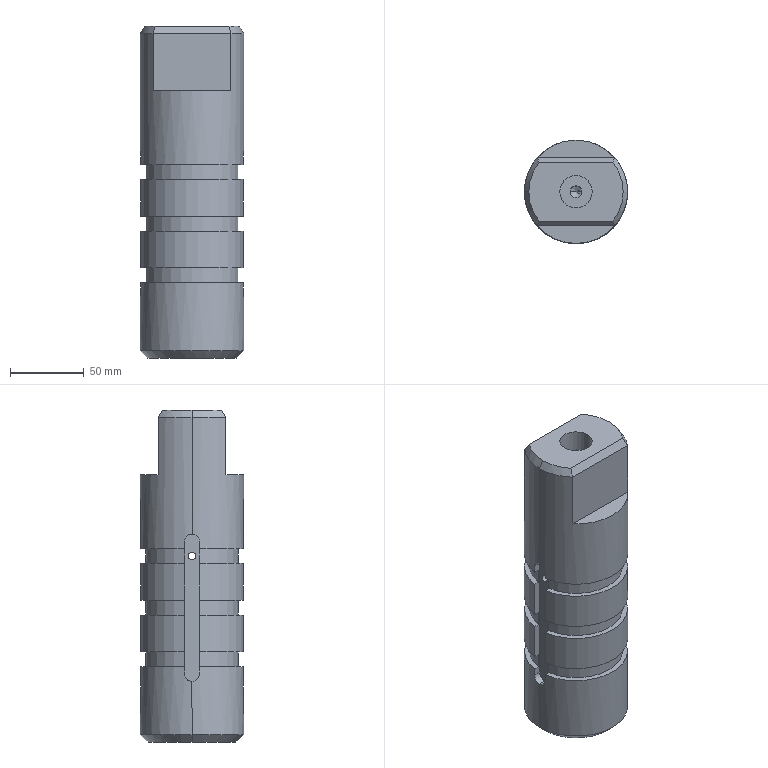Part | SolidWorks | features ICE 6, Chamfer 3, Extrusion 1, HoleWzd 1, LPattern 1 | 1 solid | 62 faces | box 70 x 70 x 225 mm | volume 782460 mm3 | cylinder 28 | plane 27 | cone 7 | commonest cylinder face diameters 70 x8 10 x6 63 x6 5 x4 8 x2 22 x2